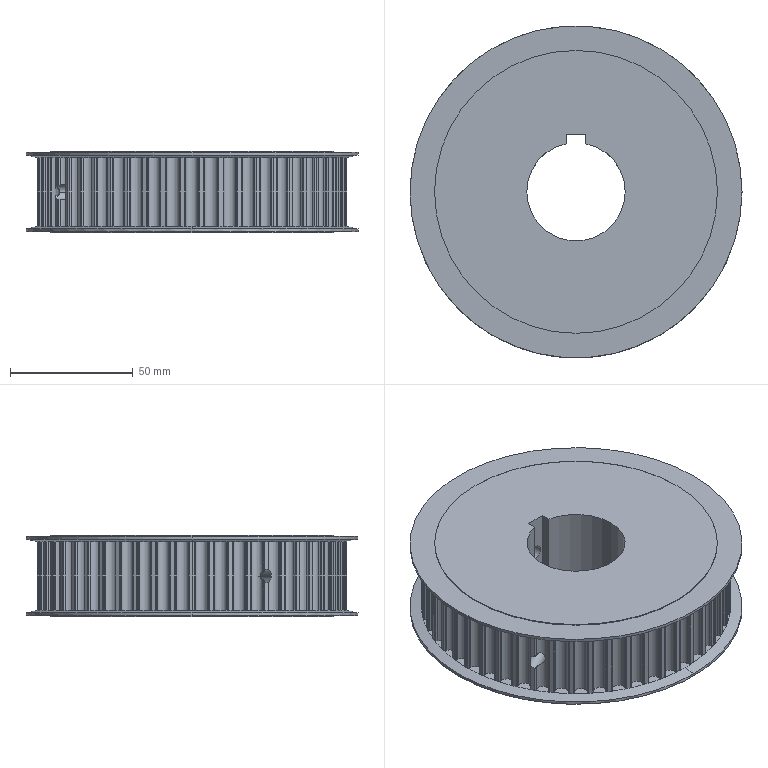Part | SolidWorks | features BaseBody 1 | 1 solid | 484 faces | box 135 x 135 x 33 mm | volume 349541 mm3 | cylinder 269 | plane 211 | cone 4 | commonest cylinder face diameters 0.81 x127 5.184 x75 125.95 x52 6 x4 115 x4 135 x4